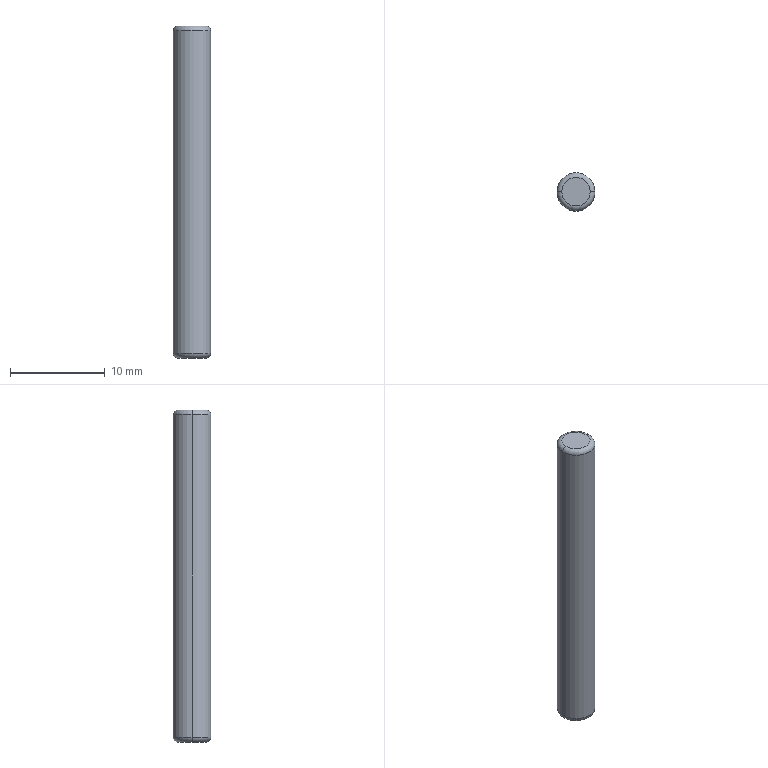Part | SolidWorks | features Extrusion 1, Fillet 1 | 1 solid | 8 faces | box 4 x 4 x 35 mm | volume 438.55 mm3 | torus 4 | cylinder 2 | plane 2 | commonest cylinder face diameters 4 x2
STEP:
#1=CARTESIAN_POINT('',(-1.5,0.,0.));
#2=VERTEX_POINT('',#1);
#3=CARTESIAN_POINT('',(1.5,0.,0.));
#4=VERTEX_POINT('',#3);
#5=CARTESIAN_POINT('',(0.,0.,0.));
#6=DIRECTION('',(0.,0.,-1.));
#7=DIRECTION('',(1.,0.,0.));
#8=AXIS2_PLACEMENT_3D('',#5,#6,#7);
#9=CIRCLE('',#8,1.5);
#10=EDGE_CURVE('',#2,#4,#9,.T.);
#11=ORIENTED_EDGE('',*,*,#10,.F.);
#12=CARTESIAN_POINT('',(-2.,0.,0.5));
#13=VERTEX_POINT('',#12);
#14=CARTESIAN_POINT('',(-1.5,0.,0.5));
#15=DIRECTION('',(0.,1.,0.));
#16=DIRECTION('',(-1.,0.,0.));
#17=AXIS2_PLACEMENT_3D('',#14,#15,#16);
#18=CIRCLE('',#17,0.5);
#19=EDGE_CURVE('',#2,#13,#18,.T.);
#20=ORIENTED_EDGE('',*,*,#19,.T.);
#21=CARTESIAN_POINT('',(2.,0.,0.5));
#22=VERTEX_POINT('',#21);
#23=CARTESIAN_POINT('',(0.,0.,0.5));
#24=DIRECTION('',(0.,0.,1.));
#25=DIRECTION('',(1.,0.,0.));
#26=AXIS2_PLACEMENT_3D('',#23,#24,#25);
#27=CIRCLE('',#26,2.);
#28=EDGE_CURVE('',#22,#13,#27,.T.);
#29=ORIENTED_EDGE('',*,*,#28,.F.);
#30=CARTESIAN_POINT('',(1.5,0.,0.5));
#31=DIRECTION('',(0.,-1.,0.));
#32=DIRECTION('',(0.,0.,-1.));
#33=AXIS2_PLACEMENT_3D('',#30,#31,#32);
#34=CIRCLE('',#33,0.5);
#35=EDGE_CURVE('',#4,#22,#34,.T.);
#36=ORIENTED_EDGE('',*,*,#35,.F.);
#37=EDGE_LOOP('',(#11,#20,#29,#36));
#38=FACE_OUTER_BOUND('',#37,.T.);
#39=CARTESIAN_POINT('',(0.,0.,0.5));
#40=DIRECTION('',(0.,0.,1.));
#41=DIRECTION('',(1.,0.,0.));
#42=AXIS2_PLACEMENT_3D('',#39,#40,#41);
#43=TOROIDAL_SURFACE('',#42,1.5,0.5);
#44=ADVANCED_FACE('',(#38),#43,.T.);
#45=CARTESIAN_POINT('',(-2.,0.,34.5));
#46=VERTEX_POINT('',#45);
#47=CARTESIAN_POINT('',(2.,0.,34.5));
#48=VERTEX_POINT('',#47);
#49=CARTESIAN_POINT('',(0.,0.,34.5));
#50=DIRECTION('',(0.,0.,-1.));
#51=DIRECTION('',(1.,0.,0.));
#52=AXIS2_PLACEMENT_3D('',#49,#50,#51);
#53=CIRCLE('',#52,2.);
#54=EDGE_CURVE('',#46,#48,#53,.T.);
#55=ORIENTED_EDGE('',*,*,#54,.F.);
#56=CARTESIAN_POINT('',(-1.5,0.,35.));
#57=VERTEX_POINT('',#56);
#58=CARTESIAN_POINT('',(-1.5,0.,34.5));
#59=DIRECTION('',(0.,1.,0.));
#60=DIRECTION('',(-1.,0.,0.));
#61=AXIS2_PLACEMENT_3D('',#58,#59,#60);
#62=CIRCLE('',#61,0.5);
#63=EDGE_CURVE('',#46,#57,#62,.T.);
#64=ORIENTED_EDGE('',*,*,#63,.T.);
#65=CARTESIAN_POINT('',(1.5,0.,35.));
#66=VERTEX_POINT('',#65);
#67=CARTESIAN_POINT('',(0.,0.,35.));
#68=DIRECTION('',(0.,0.,1.));
#69=DIRECTION('',(1.,0.,0.));
#70=AXIS2_PLACEMENT_3D('',#67,#68,#69);
#71=CIRCLE('',#70,1.5);
#72=EDGE_CURVE('',#66,#57,#71,.T.);
#73=ORIENTED_EDGE('',*,*,#72,.F.);
#74=CARTESIAN_POINT('',(1.5,0.,34.5));
#75=DIRECTION('',(0.,-1.,0.));
#76=DIRECTION('',(0.,0.,-1.));
#77=AXIS2_PLACEMENT_3D('',#74,#75,#76);
#78=CIRCLE('',#77,0.5);
#79=EDGE_CURVE('',#48,#66,#78,.T.);
#80=ORIENTED_EDGE('',*,*,#79,.F.);
#81=EDGE_LOOP('',(#55,#64,#73,#80));
#82=FACE_OUTER_BOUND('',#81,.T.);
#83=CARTESIAN_POINT('',(0.,0.,34.5));
#84=DIRECTION('',(0.,0.,1.));
#85=DIRECTION('',(1.,0.,0.));
#86=AXIS2_PLACEMENT_3D('',#83,#84,#85);
#87=TOROIDAL_SURFACE('',#86,1.5,0.5);
#88=ADVANCED_FACE('',(#82),#87,.T.);
#89=ORIENTED_EDGE('',*,*,#54,.T.);
#90=CARTESIAN_POINT('',(2.,0.,35.));
#91=DIRECTION('',(0.,0.,-1.));
#92=VECTOR('',#91,1000.);
#93=LINE('',#90,#92);
#94=EDGE_CURVE('',#48,#22,#93,.T.);
#95=ORIENTED_EDGE('',*,*,#94,.T.);
#96=ORIENTED_EDGE('',*,*,#28,.T.);
#97=CARTESIAN_POINT('',(-2.,0.,35.));
#98=DIRECTION('',(0.,0.,-1.));
#99=VECTOR('',#98,1000.);
#100=LINE('',#97,#99);
#101=EDGE_CURVE('',#46,#13,#100,.T.);
#102=ORIENTED_EDGE('',*,*,#101,.F.);
#103=EDGE_LOOP('',(#89,#95,#96,#102));
#104=FACE_OUTER_BOUND('',#103,.T.);
#105=CARTESIAN_POINT('',(0.,0.,35.));
#106=DIRECTION('',(0.,0.,-1.));
#107=DIRECTION('',(-1.,0.,0.));
#108=AXIS2_PLACEMENT_3D('',#105,#106,#107);
#109=CYLINDRICAL_SURFACE('',#108,2.);
#110=ADVANCED_FACE('',(#104),#109,.T.);
#111=ORIENTED_EDGE('',*,*,#94,.F.);
#112=CARTESIAN_POINT('',(0.,0.,34.5));
#113=DIRECTION('',(0.,0.,-1.));
#114=DIRECTION('',(1.,0.,0.));
#115=AXIS2_PLACEMENT_3D('',#112,#113,#114);
#116=CIRCLE('',#115,2.);
#117=EDGE_CURVE('',#48,#46,#116,.T.);
#118=ORIENTED_EDGE('',*,*,#117,.T.);
#119=ORIENTED_EDGE('',*,*,#101,.T.);
#120=CARTESIAN_POINT('',(0.,0.,0.5));
#121=DIRECTION('',(0.,0.,1.));
#122=DIRECTION('',(1.,0.,0.));
#123=AXIS2_PLACEMENT_3D('',#120,#121,#122);
#124=CIRCLE('',#123,2.);
#125=EDGE_CURVE('',#13,#22,#124,.T.);
#126=ORIENTED_EDGE('',*,*,#125,.T.);
#127=EDGE_LOOP('',(#111,#118,#119,#126));
#128=FACE_OUTER_BOUND('',#127,.T.);
#129=CARTESIAN_POINT('',(0.,0.,35.));
#130=DIRECTION('',(0.,0.,-1.));
#131=DIRECTION('',(-1.,0.,0.));
#132=AXIS2_PLACEMENT_3D('',#129,#130,#131);
#133=CYLINDRICAL_SURFACE('',#132,2.);
#134=ADVANCED_FACE('',(#128),#133,.T.);
#135=ORIENTED_EDGE('',*,*,#72,.T.);
#136=CARTESIAN_POINT('',(0.,0.,35.));
#137=DIRECTION('',(0.,0.,1.));
#138=DIRECTION('',(1.,0.,0.));
#139=AXIS2_PLACEMENT_3D('',#136,#137,#138);
#140=CIRCLE('',#139,1.5);
#141=EDGE_CURVE('',#57,#66,#140,.T.);
#142=ORIENTED_EDGE('',*,*,#141,.T.);
#143=EDGE_LOOP('',(#135,#142));
#144=FACE_OUTER_BOUND('',#143,.T.);
#145=CARTESIAN_POINT('',(0.,0.,35.));
#146=DIRECTION('',(0.,0.,1.));
#147=DIRECTION('',(1.,0.,0.));
#148=AXIS2_PLACEMENT_3D('',#145,#146,#147);
#149=PLANE('',#148);
#150=ADVANCED_FACE('',(#144),#149,.T.);
#151=CARTESIAN_POINT('',(0.,0.,0.));
#152=DIRECTION('',(0.,0.,-1.));
#153=DIRECTION('',(1.,0.,0.));
#154=AXIS2_PLACEMENT_3D('',#151,#152,#153);
#155=CIRCLE('',#154,1.5);
#156=EDGE_CURVE('',#4,#2,#155,.T.);
#157=ORIENTED_EDGE('',*,*,#156,.T.);
#158=ORIENTED_EDGE('',*,*,#10,.T.);
#159=EDGE_LOOP('',(#157,#158));
#160=FACE_OUTER_BOUND('',#159,.T.);
#161=CARTESIAN_POINT('',(0.,0.,0.));
#162=DIRECTION('',(0.,0.,1.));
#163=DIRECTION('',(1.,0.,0.));
#164=AXIS2_PLACEMENT_3D('',#161,#162,#163);
#165=PLANE('',#164);
#166=ADVANCED_FACE('',(#160),#165,.F.);
#167=ORIENTED_EDGE('',*,*,#63,.F.);
#168=ORIENTED_EDGE('',*,*,#117,.F.);
#169=ORIENTED_EDGE('',*,*,#79,.T.);
#170=ORIENTED_EDGE('',*,*,#141,.F.);
#171=EDGE_LOOP('',(#167,#168,#169,#170));
#172=FACE_OUTER_BOUND('',#171,.T.);
#173=CARTESIAN_POINT('',(0.,0.,34.5));
#174=DIRECTION('',(0.,0.,1.));
#175=DIRECTION('',(1.,0.,0.));
#176=AXIS2_PLACEMENT_3D('',#173,#174,#175);
#177=TOROIDAL_SURFACE('',#176,1.5,0.5);
#178=ADVANCED_FACE('',(#172),#177,.T.);
#179=ORIENTED_EDGE('',*,*,#19,.F.);
#180=ORIENTED_EDGE('',*,*,#156,.F.);
#181=ORIENTED_EDGE('',*,*,#35,.T.);
#182=ORIENTED_EDGE('',*,*,#125,.F.);
#183=EDGE_LOOP('',(#179,#180,#181,#182));
#184=FACE_OUTER_BOUND('',#183,.T.);
#185=CARTESIAN_POINT('',(0.,0.,0.5));
#186=DIRECTION('',(0.,0.,1.));
#187=DIRECTION('',(1.,0.,0.));
#188=AXIS2_PLACEMENT_3D('',#185,#186,#187);
#189=TOROIDAL_SURFACE('',#188,1.5,0.5);
#190=ADVANCED_FACE('',(#184),#189,.T.);
#191=CLOSED_SHELL('',(#44,#88,#110,#134,#150,#166,#178,#190));
#192=MANIFOLD_SOLID_BREP('',#191);
#193=CARTESIAN_POINT('',(0.,0.,0.));
#194=DIRECTION('',(0.,0.,1.));
#195=DIRECTION('',(1.,0.,0.));
#196=AXIS2_PLACEMENT_3D('',#193,#194,#195);
#197=(LENGTH_UNIT()NAMED_UNIT(*)SI_UNIT(.MILLI.,.METRE.));
#198=UNCERTAINTY_MEASURE_WITH_UNIT(LENGTH_MEASURE(0.00001),#197,'','');
#199=(NAMED_UNIT(*)PLANE_ANGLE_UNIT()SI_UNIT($,.RADIAN.));
#200=(NAMED_UNIT(*)SI_UNIT($,.STERADIAN.)SOLID_ANGLE_UNIT());
#201=(GEOMETRIC_REPRESENTATION_CONTEXT(3)GLOBAL_UNCERTAINTY_ASSIGNED_CONTEXT((#198))GLOBAL_UNIT_ASSIGNED_CONTEXT((#197,#199,#200))REPRESENTATION_CONTEXT('',''));
#202=ADVANCED_BREP_SHAPE_REPRESENTATION('',(#192,#196),#201);